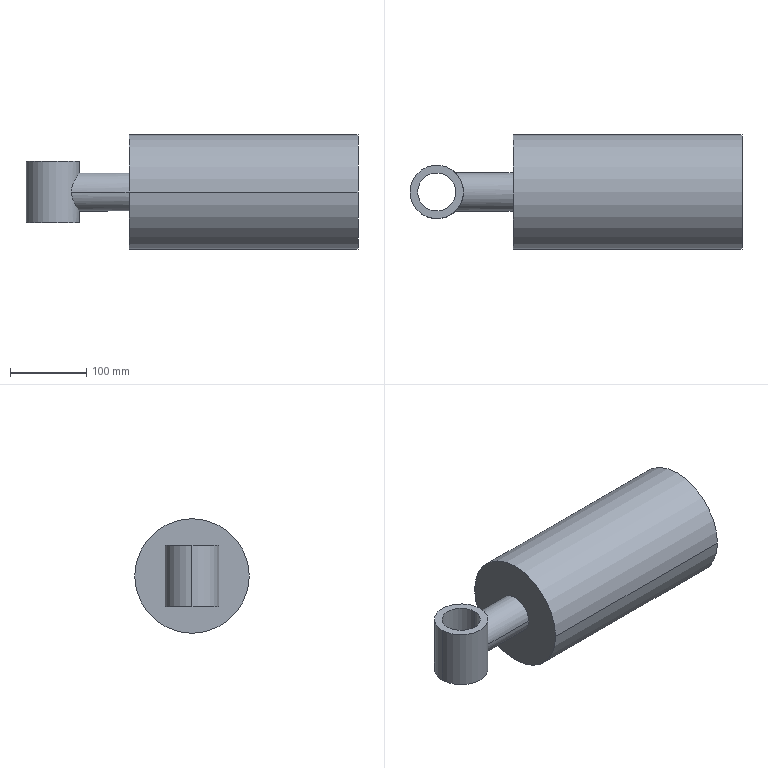Part | SolidWorks | 1 solid | 18 faces | box 435 x 150 x 150 mm | volume 3088587 mm3 | cylinder 12 | plane 6 | commonest cylinder face diameters 50 x4 40 x2 70 x2 110 x2 150 x2
STEP:
#1=CARTESIAN_POINT('',(400.,-75.,0.));
#2=VERTEX_POINT('',#1);
#3=CARTESIAN_POINT('',(400.,75.,0.));
#4=VERTEX_POINT('',#3);
#5=CARTESIAN_POINT('',(400.,0.,0.));
#6=DIRECTION('',(-1.,0.,0.));
#7=DIRECTION('',(0.,-1.,0.));
#8=AXIS2_PLACEMENT_3D('',#5,#6,#7);
#9=CIRCLE('',#8,75.);
#10=EDGE_CURVE('',#2,#4,#9,.T.);
#11=ORIENTED_EDGE('',*,*,#10,.T.);
#12=CARTESIAN_POINT('',(100.,75.,0.));
#13=VERTEX_POINT('',#12);
#14=CARTESIAN_POINT('',(0.,75.,0.));
#15=DIRECTION('',(-1.,0.,0.));
#16=VECTOR('',#15,1000.);
#17=LINE('',#14,#16);
#18=EDGE_CURVE('',#4,#13,#17,.T.);
#19=ORIENTED_EDGE('',*,*,#18,.T.);
#20=CARTESIAN_POINT('',(100.,-75.,0.));
#21=VERTEX_POINT('',#20);
#22=CARTESIAN_POINT('',(100.,0.,0.));
#23=DIRECTION('',(-1.,0.,0.));
#24=DIRECTION('',(0.,-1.,0.));
#25=AXIS2_PLACEMENT_3D('',#22,#23,#24);
#26=CIRCLE('',#25,75.);
#27=EDGE_CURVE('',#21,#13,#26,.T.);
#28=ORIENTED_EDGE('',*,*,#27,.F.);
#29=CARTESIAN_POINT('',(0.,-75.,0.));
#30=DIRECTION('',(-1.,0.,0.));
#31=VECTOR('',#30,1000.);
#32=LINE('',#29,#31);
#33=EDGE_CURVE('',#2,#21,#32,.T.);
#34=ORIENTED_EDGE('',*,*,#33,.F.);
#35=EDGE_LOOP('',(#11,#19,#28,#34));
#36=FACE_OUTER_BOUND('',#35,.T.);
#37=CARTESIAN_POINT('',(0.,0.,0.));
#38=DIRECTION('',(-1.,0.,0.));
#39=DIRECTION('',(0.,-1.,0.));
#40=AXIS2_PLACEMENT_3D('',#37,#38,#39);
#41=CYLINDRICAL_SURFACE('',#40,75.);
#42=ADVANCED_FACE('',(#36),#41,.T.);
#43=CARTESIAN_POINT('',(400.,20.,0.));
#44=VERTEX_POINT('',#43);
#45=CARTESIAN_POINT('',(400.,-20.,0.));
#46=VERTEX_POINT('',#45);
#47=CARTESIAN_POINT('',(400.,0.,0.));
#48=DIRECTION('',(-1.,0.,0.));
#49=DIRECTION('',(0.,-1.,0.));
#50=AXIS2_PLACEMENT_3D('',#47,#48,#49);
#51=CIRCLE('',#50,20.);
#52=EDGE_CURVE('',#44,#46,#51,.T.);
#53=ORIENTED_EDGE('',*,*,#52,.F.);
#54=CARTESIAN_POINT('',(380.,20.,0.));
#55=VERTEX_POINT('',#54);
#56=CARTESIAN_POINT('',(0.,20.,0.));
#57=DIRECTION('',(-1.,0.,0.));
#58=VECTOR('',#57,1000.);
#59=LINE('',#56,#58);
#60=EDGE_CURVE('',#44,#55,#59,.T.);
#61=ORIENTED_EDGE('',*,*,#60,.T.);
#62=CARTESIAN_POINT('',(380.,-20.,0.));
#63=VERTEX_POINT('',#62);
#64=CARTESIAN_POINT('',(380.,0.,0.));
#65=DIRECTION('',(-1.,0.,0.));
#66=DIRECTION('',(0.,-1.,0.));
#67=AXIS2_PLACEMENT_3D('',#64,#65,#66);
#68=CIRCLE('',#67,20.);
#69=EDGE_CURVE('',#55,#63,#68,.T.);
#70=ORIENTED_EDGE('',*,*,#69,.T.);
#71=CARTESIAN_POINT('',(0.,-20.,0.));
#72=DIRECTION('',(-1.,0.,0.));
#73=VECTOR('',#72,1000.);
#74=LINE('',#71,#73);
#75=EDGE_CURVE('',#46,#63,#74,.T.);
#76=ORIENTED_EDGE('',*,*,#75,.F.);
#77=EDGE_LOOP('',(#53,#61,#70,#76));
#78=FACE_OUTER_BOUND('',#77,.T.);
#79=CARTESIAN_POINT('',(0.,0.,0.));
#80=DIRECTION('',(-1.,0.,0.));
#81=DIRECTION('',(0.,-1.,0.));
#82=AXIS2_PLACEMENT_3D('',#79,#80,#81);
#83=CYLINDRICAL_SURFACE('',#82,20.);
#84=ADVANCED_FACE('',(#78),#83,.F.);
#85=CARTESIAN_POINT('',(380.,55.,0.));
#86=VERTEX_POINT('',#85);
#87=CARTESIAN_POINT('',(380.,-55.,0.));
#88=VERTEX_POINT('',#87);
#89=CARTESIAN_POINT('',(380.,0.,0.));
#90=DIRECTION('',(-1.,0.,0.));
#91=DIRECTION('',(0.,-1.,0.));
#92=AXIS2_PLACEMENT_3D('',#89,#90,#91);
#93=CIRCLE('',#92,55.);
#94=EDGE_CURVE('',#86,#88,#93,.T.);
#95=ORIENTED_EDGE('',*,*,#94,.F.);
#96=CARTESIAN_POINT('',(120.,55.,0.));
#97=VERTEX_POINT('',#96);
#98=CARTESIAN_POINT('',(0.,55.,0.));
#99=DIRECTION('',(-1.,0.,0.));
#100=VECTOR('',#99,1000.);
#101=LINE('',#98,#100);
#102=EDGE_CURVE('',#86,#97,#101,.T.);
#103=ORIENTED_EDGE('',*,*,#102,.T.);
#104=CARTESIAN_POINT('',(120.,-55.,0.));
#105=VERTEX_POINT('',#104);
#106=CARTESIAN_POINT('',(120.,0.,0.));
#107=DIRECTION('',(-1.,0.,0.));
#108=DIRECTION('',(0.,-1.,0.));
#109=AXIS2_PLACEMENT_3D('',#106,#107,#108);
#110=CIRCLE('',#109,55.);
#111=EDGE_CURVE('',#97,#105,#110,.T.);
#112=ORIENTED_EDGE('',*,*,#111,.T.);
#113=CARTESIAN_POINT('',(0.,-55.,0.));
#114=DIRECTION('',(-1.,0.,0.));
#115=VECTOR('',#114,1000.);
#116=LINE('',#113,#115);
#117=EDGE_CURVE('',#88,#105,#116,.T.);
#118=ORIENTED_EDGE('',*,*,#117,.F.);
#119=EDGE_LOOP('',(#95,#103,#112,#118));
#120=FACE_OUTER_BOUND('',#119,.T.);
#121=CARTESIAN_POINT('',(0.,0.,0.));
#122=DIRECTION('',(-1.,0.,0.));
#123=DIRECTION('',(0.,-1.,0.));
#124=AXIS2_PLACEMENT_3D('',#121,#122,#123);
#125=CYLINDRICAL_SURFACE('',#124,55.);
#126=ADVANCED_FACE('',(#120),#125,.F.);
#127=CARTESIAN_POINT('',(100.,-25.,0.));
#128=VERTEX_POINT('',#127);
#129=CARTESIAN_POINT('',(100.,25.,0.));
#130=VERTEX_POINT('',#129);
#131=CARTESIAN_POINT('',(100.,0.,0.));
#132=DIRECTION('',(-1.,0.,0.));
#133=DIRECTION('',(0.,-1.,0.));
#134=AXIS2_PLACEMENT_3D('',#131,#132,#133);
#135=CIRCLE('',#134,25.);
#136=EDGE_CURVE('',#128,#130,#135,.T.);
#137=ORIENTED_EDGE('',*,*,#136,.T.);
#138=CARTESIAN_POINT('',(24.495,25.,0.));
#139=VERTEX_POINT('',#138);
#140=CARTESIAN_POINT('',(0.,25.,0.));
#141=DIRECTION('',(-1.,0.,0.));
#142=VECTOR('',#141,1000.);
#143=LINE('',#140,#142);
#144=EDGE_CURVE('',#130,#139,#143,.T.);
#145=ORIENTED_EDGE('',*,*,#144,.T.);
#146=CARTESIAN_POINT('',(35.,0.,25.));
#147=VERTEX_POINT('',#146);
#148=CARTESIAN_POINT('',(24.495,25.,0.));
#149=CARTESIAN_POINT('',(24.495,25.,0.8465));
#150=CARTESIAN_POINT('',(24.539,24.957,1.695));
#151=CARTESIAN_POINT('',(24.671,24.826,2.973));
#152=CARTESIAN_POINT('',(24.726,24.772,3.398));
#153=CARTESIAN_POINT('',(24.855,24.642,4.235));
#154=CARTESIAN_POINT('',(24.929,24.567,4.649));
#155=CARTESIAN_POINT('',(25.178,24.313,5.879));
#156=CARTESIAN_POINT('',(25.379,24.105,6.682));
#157=CARTESIAN_POINT('',(25.838,23.612,8.257));
#158=CARTESIAN_POINT('',(26.097,23.326,9.031));
#159=CARTESIAN_POINT('',(26.925,22.377,11.264));
#160=CARTESIAN_POINT('',(27.546,21.62,12.651));
#161=CARTESIAN_POINT('',(28.516,20.301,14.612));
#162=CARTESIAN_POINT('',(28.847,19.829,15.245));
#163=CARTESIAN_POINT('',(29.513,18.825,16.47));
#164=CARTESIAN_POINT('',(29.844,18.297,17.054));
#165=CARTESIAN_POINT('',(30.82,16.636,18.728));
#166=CARTESIAN_POINT('',(31.451,15.426,19.739));
#167=CARTESIAN_POINT('',(32.327,13.436,21.098));
#168=CARTESIAN_POINT('',(32.608,12.74,21.526));
#169=CARTESIAN_POINT('',(33.13,11.312,22.309));
#170=CARTESIAN_POINT('',(33.372,10.579,22.666));
#171=CARTESIAN_POINT('',(33.814,9.07,23.311));
#172=CARTESIAN_POINT('',(34.013,8.294,23.599));
#173=CARTESIAN_POINT('',(34.363,6.698,24.1));
#174=CARTESIAN_POINT('',(34.514,5.872,24.315));
#175=CARTESIAN_POINT('',(34.876,3.386,24.827));
#176=CARTESIAN_POINT('',(35.,1.705,25.));
#177=CARTESIAN_POINT('',(35.,0.,25.));
#178=B_SPLINE_CURVE_WITH_KNOTS('',3,(#148,#149,#150,#151,#152,#153,#154,#155,#156,#157,#158,#159,#160,#161,#162,#163,#164,#165,#166,#167,#168,#169,#170,#171,#172,#173,#174,#175,#176,#177),.UNSPECIFIED.,.F.,.F.,(4,2,2,2,2,2,2,2,2,2,2,2,2,2,4),(0.08125,0.08378,0.08505,0.08632,0.08886,0.09139,0.09647,0.099,0.1015,0.1066,0.1091,0.1117,0.1142,0.1168,0.1218),.UNSPECIFIED.);
#179=EDGE_CURVE('',#139,#147,#178,.T.);
#180=ORIENTED_EDGE('',*,*,#179,.T.);
#181=CARTESIAN_POINT('',(24.495,-25.,0.));
#182=VERTEX_POINT('',#181);
#183=CARTESIAN_POINT('',(35.,0.,25.));
#184=CARTESIAN_POINT('',(35.,-0.4259,25.));
#185=CARTESIAN_POINT('',(34.992,-0.8533,24.989));
#186=CARTESIAN_POINT('',(34.961,-1.711,24.945));
#187=CARTESIAN_POINT('',(34.937,-2.14,24.912));
#188=CARTESIAN_POINT('',(34.844,-3.414,24.781));
#189=CARTESIAN_POINT('',(34.751,-4.25,24.651));
#190=CARTESIAN_POINT('',(34.51,-5.897,24.309));
#191=CARTESIAN_POINT('',(34.361,-6.709,24.098));
#192=CARTESIAN_POINT('',(34.097,-7.908,23.72));
#193=CARTESIAN_POINT('',(34.003,-8.306,23.584));
#194=CARTESIAN_POINT('',(33.802,-9.088,23.293));
#195=CARTESIAN_POINT('',(33.696,-9.473,23.139));
#196=CARTESIAN_POINT('',(33.14,-11.367,22.327));
#197=CARTESIAN_POINT('',(32.614,-12.786,21.544));
#198=CARTESIAN_POINT('',(31.733,-14.784,20.177));
#199=CARTESIAN_POINT('',(31.426,-15.422,19.692));
#200=CARTESIAN_POINT('',(30.8,-16.639,18.676));
#201=CARTESIAN_POINT('',(30.478,-17.219,18.142));
#202=CARTESIAN_POINT('',(29.827,-18.325,17.024));
#203=CARTESIAN_POINT('',(29.496,-18.851,16.44));
#204=CARTESIAN_POINT('',(28.833,-19.85,15.218));
#205=CARTESIAN_POINT('',(28.5,-20.323,14.58));
#206=CARTESIAN_POINT('',(27.53,-21.641,12.616));
#207=CARTESIAN_POINT('',(26.912,-22.393,11.231));
#208=CARTESIAN_POINT('',(26.091,-23.333,9.012));
#209=CARTESIAN_POINT('',(25.836,-23.614,8.249));
#210=CARTESIAN_POINT('',(25.49,-23.985,7.063));
#211=CARTESIAN_POINT('',(25.381,-24.1,6.661));
#212=CARTESIAN_POINT('',(25.182,-24.308,5.855));
#213=CARTESIAN_POINT('',(25.091,-24.402,5.45));
#214=CARTESIAN_POINT('',(24.844,-24.655,4.224));
#215=CARTESIAN_POINT('',(24.715,-24.783,3.397));
#216=CARTESIAN_POINT('',(24.584,-24.912,2.137));
#217=CARTESIAN_POINT('',(24.551,-24.945,1.714));
#218=CARTESIAN_POINT('',(24.506,-24.989,0.8617));
#219=CARTESIAN_POINT('',(24.495,-25.,0.4306));
#220=CARTESIAN_POINT('',(24.495,-25.,0.));
#221=B_SPLINE_CURVE_WITH_KNOTS('',3,(#183,#184,#185,#186,#187,#188,#189,#190,#191,#192,#193,#194,#195,#196,#197,#198,#199,#200,#201,#202,#203,#204,#205,#206,#207,#208,#209,#210,#211,#212,#213,#214,#215,#216,#217,#218,#219,#220),.UNSPECIFIED.,.F.,.F.,(4,2,2,2,2,2,2,2,2,2,2,2,2,2,2,2,2,2,4),(0.1218,0.1231,0.1244,0.1269,0.1294,0.1307,0.132,0.137,0.1396,0.1421,0.1446,0.1472,0.1522,0.1548,0.156,0.1573,0.1598,0.1611,0.1624),.UNSPECIFIED.);
#222=EDGE_CURVE('',#147,#182,#221,.T.);
#223=ORIENTED_EDGE('',*,*,#222,.T.);
#224=CARTESIAN_POINT('',(0.,-25.,0.));
#225=DIRECTION('',(-1.,0.,0.));
#226=VECTOR('',#225,1000.);
#227=LINE('',#224,#226);
#228=EDGE_CURVE('',#128,#182,#227,.T.);
#229=ORIENTED_EDGE('',*,*,#228,.F.);
#230=EDGE_LOOP('',(#137,#145,#180,#223,#229));
#231=FACE_OUTER_BOUND('',#230,.T.);
#232=CARTESIAN_POINT('',(0.,0.,0.));
#233=DIRECTION('',(-1.,0.,0.));
#234=DIRECTION('',(0.,-1.,0.));
#235=AXIS2_PLACEMENT_3D('',#232,#233,#234);
#236=CYLINDRICAL_SURFACE('',#235,25.);
#237=ADVANCED_FACE('',(#231),#236,.T.);
#238=CARTESIAN_POINT('',(-25.,0.,40.));
#239=VERTEX_POINT('',#238);
#240=CARTESIAN_POINT('',(25.,0.,40.));
#241=VERTEX_POINT('',#240);
#242=CARTESIAN_POINT('',(0.,0.,40.));
#243=DIRECTION('',(0.,0.,1.));
#244=DIRECTION('',(1.,0.,0.));
#245=AXIS2_PLACEMENT_3D('',#242,#243,#244);
#246=CIRCLE('',#245,25.);
#247=EDGE_CURVE('',#239,#241,#246,.T.);
#248=ORIENTED_EDGE('',*,*,#247,.T.);
#249=CARTESIAN_POINT('',(25.,0.,-40.));
#250=VERTEX_POINT('',#249);
#251=CARTESIAN_POINT('',(25.,0.,40.));
#252=DIRECTION('',(0.,0.,-1.));
#253=VECTOR('',#252,1000.);
#254=LINE('',#251,#253);
#255=EDGE_CURVE('',#241,#250,#254,.T.);
#256=ORIENTED_EDGE('',*,*,#255,.T.);
#257=CARTESIAN_POINT('',(-25.,0.,-40.));
#258=VERTEX_POINT('',#257);
#259=CARTESIAN_POINT('',(0.,0.,-40.));
#260=DIRECTION('',(0.,0.,1.));
#261=DIRECTION('',(1.,0.,0.));
#262=AXIS2_PLACEMENT_3D('',#259,#260,#261);
#263=CIRCLE('',#262,25.);
#264=EDGE_CURVE('',#258,#250,#263,.T.);
#265=ORIENTED_EDGE('',*,*,#264,.F.);
#266=CARTESIAN_POINT('',(-25.,0.,40.));
#267=DIRECTION('',(0.,0.,-1.));
#268=VECTOR('',#267,1000.);
#269=LINE('',#266,#268);
#270=EDGE_CURVE('',#239,#258,#269,.T.);
#271=ORIENTED_EDGE('',*,*,#270,.F.);
#272=EDGE_LOOP('',(#248,#256,#265,#271));
#273=FACE_OUTER_BOUND('',#272,.T.);
#274=CARTESIAN_POINT('',(0.,0.,40.));
#275=DIRECTION('',(0.,0.,-1.));
#276=DIRECTION('',(-1.,0.,0.));
#277=AXIS2_PLACEMENT_3D('',#274,#275,#276);
#278=CYLINDRICAL_SURFACE('',#277,25.);
#279=ADVANCED_FACE('',(#273),#278,.F.);
#280=CARTESIAN_POINT('',(35.,0.,40.));
#281=VERTEX_POINT('',#280);
#282=CARTESIAN_POINT('',(-35.,0.,40.));
#283=VERTEX_POINT('',#282);
#284=CARTESIAN_POINT('',(0.,0.,40.));
#285=DIRECTION('',(0.,0.,1.));
#286=DIRECTION('',(1.,0.,0.));
#287=AXIS2_PLACEMENT_3D('',#284,#285,#286);
#288=CIRCLE('',#287,35.);
#289=EDGE_CURVE('',#281,#283,#288,.T.);
#290=ORIENTED_EDGE('',*,*,#289,.F.);
#291=CARTESIAN_POINT('',(35.,0.,40.));
#292=DIRECTION('',(0.,0.,-1.));
#293=VECTOR('',#292,1000.);
#294=LINE('',#291,#293);
#295=EDGE_CURVE('',#281,#147,#294,.T.);
#296=ORIENTED_EDGE('',*,*,#295,.T.);
#297=ORIENTED_EDGE('',*,*,#179,.F.);
#298=CARTESIAN_POINT('',(35.,0.,-25.));
#299=VERTEX_POINT('',#298);
#300=CARTESIAN_POINT('',(35.,0.,-25.));
#301=CARTESIAN_POINT('',(35.,1.707,-25.));
#302=CARTESIAN_POINT('',(34.876,3.392,-24.827));
#303=CARTESIAN_POINT('',(34.573,5.47,-24.398));
#304=CARTESIAN_POINT('',(34.504,5.885,-24.301));
#305=CARTESIAN_POINT('',(34.355,6.702,-24.089));
#306=CARTESIAN_POINT('',(34.274,7.106,-23.973));
#307=CARTESIAN_POINT('',(34.011,8.3,-23.597));
#308=CARTESIAN_POINT('',(33.812,9.076,-23.309));
#309=CARTESIAN_POINT('',(33.369,10.589,-22.662));
#310=CARTESIAN_POINT('',(33.125,11.327,-22.302));
#311=CARTESIAN_POINT('',(32.599,12.762,-21.513));
#312=CARTESIAN_POINT('',(32.321,13.449,-21.089));
#313=CARTESIAN_POINT('',(31.447,15.432,-19.733));
#314=CARTESIAN_POINT('',(30.814,16.648,-18.718));
#315=CARTESIAN_POINT('',(29.498,18.882,-16.462));
#316=CARTESIAN_POINT('',(28.832,19.873,-15.249));
#317=CARTESIAN_POINT('',(27.864,21.187,-13.294));
#318=CARTESIAN_POINT('',(27.547,21.596,-12.619));
#319=CARTESIAN_POINT('',(26.934,22.356,-11.217));
#320=CARTESIAN_POINT('',(26.636,22.709,-10.487));
#321=CARTESIAN_POINT('',(25.81,23.655,-8.25));
#322=CARTESIAN_POINT('',(25.341,24.147,-6.691));
#323=CARTESIAN_POINT('',(24.926,24.571,-4.631));
#324=CARTESIAN_POINT('',(24.851,24.646,-4.212));
#325=CARTESIAN_POINT('',(24.723,24.775,-3.373));
#326=CARTESIAN_POINT('',(24.669,24.829,-2.953));
#327=CARTESIAN_POINT('',(24.539,24.957,-1.69));
#328=CARTESIAN_POINT('',(24.495,25.,-0.8465));
#329=CARTESIAN_POINT('',(24.495,25.,0.));
#330=B_SPLINE_CURVE_WITH_KNOTS('',3,(#300,#301,#302,#303,#304,#305,#306,#307,#308,#309,#310,#311,#312,#313,#314,#315,#316,#317,#318,#319,#320,#321,#322,#323,#324,#325,#326,#327,#328,#329),.UNSPECIFIED.,.F.,.F.,(4,2,2,2,2,2,2,2,2,2,2,2,2,2,4),(0.04066,0.04573,0.047,0.04827,0.0508,0.05334,0.05588,0.06095,0.06602,0.06856,0.0711,0.07617,0.07744,0.07871,0.08125),.UNSPECIFIED.);
#331=EDGE_CURVE('',#299,#139,#330,.T.);
#332=ORIENTED_EDGE('',*,*,#331,.F.);
#333=CARTESIAN_POINT('',(35.,0.,-40.));
#334=VERTEX_POINT('',#333);
#335=CARTESIAN_POINT('',(35.,0.,40.));
#336=DIRECTION('',(0.,0.,-1.));
#337=VECTOR('',#336,1000.);
#338=LINE('',#335,#337);
#339=EDGE_CURVE('',#299,#334,#338,.T.);
#340=ORIENTED_EDGE('',*,*,#339,.T.);
#341=CARTESIAN_POINT('',(-35.,0.,-40.));
#342=VERTEX_POINT('',#341);
#343=CARTESIAN_POINT('',(0.,0.,-40.));
#344=DIRECTION('',(0.,0.,1.));
#345=DIRECTION('',(1.,0.,0.));
#346=AXIS2_PLACEMENT_3D('',#343,#344,#345);
#347=CIRCLE('',#346,35.);
#348=EDGE_CURVE('',#334,#342,#347,.T.);
#349=ORIENTED_EDGE('',*,*,#348,.T.);
#350=CARTESIAN_POINT('',(-35.,0.,40.));
#351=DIRECTION('',(0.,0.,-1.));
#352=VECTOR('',#351,1000.);
#353=LINE('',#350,#352);
#354=EDGE_CURVE('',#283,#342,#353,.T.);
#355=ORIENTED_EDGE('',*,*,#354,.F.);
#356=EDGE_LOOP('',(#290,#296,#297,#332,#340,#349,#355));
#357=FACE_OUTER_BOUND('',#356,.T.);
#358=CARTESIAN_POINT('',(0.,0.,40.));
#359=DIRECTION('',(0.,0.,-1.));
#360=DIRECTION('',(-1.,0.,0.));
#361=AXIS2_PLACEMENT_3D('',#358,#359,#360);
#362=CYLINDRICAL_SURFACE('',#361,35.);
#363=ADVANCED_FACE('',(#357),#362,.T.);
#364=ORIENTED_EDGE('',*,*,#295,.F.);
#365=CARTESIAN_POINT('',(0.,0.,40.));
#366=DIRECTION('',(0.,0.,1.));
#367=DIRECTION('',(1.,0.,0.));
#368=AXIS2_PLACEMENT_3D('',#365,#366,#367);
#369=CIRCLE('',#368,35.);
#370=EDGE_CURVE('',#283,#281,#369,.T.);
#371=ORIENTED_EDGE('',*,*,#370,.F.);
#372=ORIENTED_EDGE('',*,*,#354,.T.);
#373=CARTESIAN_POINT('',(0.,0.,-40.));
#374=DIRECTION('',(0.,0.,1.));
#375=DIRECTION('',(1.,0.,0.));
#376=AXIS2_PLACEMENT_3D('',#373,#374,#375);
#377=CIRCLE('',#376,35.);
#378=EDGE_CURVE('',#342,#334,#377,.T.);
#379=ORIENTED_EDGE('',*,*,#378,.T.);
#380=ORIENTED_EDGE('',*,*,#339,.F.);
#381=CARTESIAN_POINT('',(24.495,-25.,0.));
#382=CARTESIAN_POINT('',(24.495,-25.,-1.727));
#383=CARTESIAN_POINT('',(24.678,-24.823,-3.404));
#384=CARTESIAN_POINT('',(25.09,-24.403,-5.446));
#385=CARTESIAN_POINT('',(25.181,-24.309,-5.851));
#386=CARTESIAN_POINT('',(25.381,-24.101,-6.658));
#387=CARTESIAN_POINT('',(25.489,-23.986,-7.059));
#388=CARTESIAN_POINT('',(25.834,-23.616,-8.244));
#389=CARTESIAN_POINT('',(26.09,-23.335,-9.008));
#390=CARTESIAN_POINT('',(26.639,-22.705,-10.493));
#391=CARTESIAN_POINT('',(26.933,-22.358,-11.214));
#392=CARTESIAN_POINT('',(27.546,-21.597,-12.617));
#393=CARTESIAN_POINT('',(27.868,-21.182,-13.302));
#394=CARTESIAN_POINT('',(28.843,-19.857,-15.271));
#395=CARTESIAN_POINT('',(29.51,-18.863,-16.482));
#396=CARTESIAN_POINT('',(30.326,-17.476,-17.881));
#397=CARTESIAN_POINT('',(30.489,-17.192,-18.155));
#398=CARTESIAN_POINT('',(30.811,-16.607,-18.691));
#399=CARTESIAN_POINT('',(30.971,-16.306,-18.954));
#400=CARTESIAN_POINT('',(31.444,-15.387,-19.72));
#401=CARTESIAN_POINT('',(31.747,-14.752,-20.199));
#402=CARTESIAN_POINT('',(32.616,-12.779,-21.546));
#403=CARTESIAN_POINT('',(33.138,-11.373,-22.324));
#404=CARTESIAN_POINT('',(33.693,-9.484,-23.135));
#405=CARTESIAN_POINT('',(33.799,-9.1,-23.289));
#406=CARTESIAN_POINT('',(34.,-8.318,-23.579));
#407=CARTESIAN_POINT('',(34.095,-7.919,-23.716));
#408=CARTESIAN_POINT('',(34.359,-6.718,-24.095));
#409=CARTESIAN_POINT('',(34.508,-5.905,-24.307));
#410=CARTESIAN_POINT('',(34.75,-4.256,-24.649));
#411=CARTESIAN_POINT('',(34.843,-3.419,-24.78));
#412=CARTESIAN_POINT('',(34.968,-1.721,-24.955));
#413=CARTESIAN_POINT('',(35.,-0.8551,-25.));
#414=CARTESIAN_POINT('',(35.,0.,-25.));
#415=B_SPLINE_CURVE_WITH_KNOTS('',3,(#381,#382,#383,#384,#385,#386,#387,#388,#389,#390,#391,#392,#393,#394,#395,#396,#397,#398,#399,#400,#401,#402,#403,#404,#405,#406,#407,#408,#409,#410,#411,#412,#413,#414),.UNSPECIFIED.,.F.,.F.,(4,2,2,2,2,2,2,2,2,2,2,2,2,2,2,2,4),(0.,0.005082,0.006352,0.007623,0.01016,0.0127,0.01525,0.02033,0.0216,0.02287,0.02541,0.03049,0.03176,0.03303,0.03557,0.03811,0.04066),.UNSPECIFIED.);
#416=EDGE_CURVE('',#182,#299,#415,.T.);
#417=ORIENTED_EDGE('',*,*,#416,.F.);
#418=ORIENTED_EDGE('',*,*,#222,.F.);
#419=EDGE_LOOP('',(#364,#371,#372,#379,#380,#417,#418));
#420=FACE_OUTER_BOUND('',#419,.T.);
#421=CARTESIAN_POINT('',(0.,0.,40.));
#422=DIRECTION('',(0.,0.,-1.));
#423=DIRECTION('',(-1.,0.,0.));
#424=AXIS2_PLACEMENT_3D('',#421,#422,#423);
#425=CYLINDRICAL_SURFACE('',#424,35.);
#426=ADVANCED_FACE('',(#420),#425,.T.);
#427=ORIENTED_EDGE('',*,*,#255,.F.);
#428=CARTESIAN_POINT('',(0.,0.,40.));
#429=DIRECTION('',(0.,0.,1.));
#430=DIRECTION('',(1.,0.,0.));
#431=AXIS2_PLACEMENT_3D('',#428,#429,#430);
#432=CIRCLE('',#431,25.);
#433=EDGE_CURVE('',#241,#239,#432,.T.);
#434=ORIENTED_EDGE('',*,*,#433,.T.);
#435=ORIENTED_EDGE('',*,*,#270,.T.);
#436=CARTESIAN_POINT('',(0.,0.,-40.));
#437=DIRECTION('',(0.,0.,1.));
#438=DIRECTION('',(1.,0.,0.));
#439=AXIS2_PLACEMENT_3D('',#436,#437,#438);
#440=CIRCLE('',#439,25.);
#441=EDGE_CURVE('',#250,#258,#440,.T.);
#442=ORIENTED_EDGE('',*,*,#441,.F.);
#443=EDGE_LOOP('',(#427,#434,#435,#442));
#444=FACE_OUTER_BOUND('',#443,.T.);
#445=CARTESIAN_POINT('',(0.,0.,40.));
#446=DIRECTION('',(0.,0.,-1.));
#447=DIRECTION('',(-1.,0.,0.));
#448=AXIS2_PLACEMENT_3D('',#445,#446,#447);
#449=CYLINDRICAL_SURFACE('',#448,25.);
#450=ADVANCED_FACE('',(#444),#449,.F.);
#451=ORIENTED_EDGE('',*,*,#370,.T.);
#452=ORIENTED_EDGE('',*,*,#289,.T.);
#453=EDGE_LOOP('',(#451,#452));
#454=FACE_OUTER_BOUND('',#453,.T.);
#455=ORIENTED_EDGE('',*,*,#247,.F.);
#456=ORIENTED_EDGE('',*,*,#433,.F.);
#457=EDGE_LOOP('',(#455,#456));
#458=FACE_BOUND('',#457,.T.);
#459=CARTESIAN_POINT('',(0.,0.,40.));
#460=DIRECTION('',(0.,0.,1.));
#461=DIRECTION('',(1.,0.,0.));
#462=AXIS2_PLACEMENT_3D('',#459,#460,#461);
#463=PLANE('',#462);
#464=ADVANCED_FACE('',(#454,#458),#463,.T.);
#465=ORIENTED_EDGE('',*,*,#378,.F.);
#466=ORIENTED_EDGE('',*,*,#348,.F.);
#467=EDGE_LOOP('',(#465,#466));
#468=FACE_OUTER_BOUND('',#467,.T.);
#469=ORIENTED_EDGE('',*,*,#264,.T.);
#470=ORIENTED_EDGE('',*,*,#441,.T.);
#471=EDGE_LOOP('',(#469,#470));
#472=FACE_BOUND('',#471,.T.);
#473=CARTESIAN_POINT('',(0.,0.,-40.));
#474=DIRECTION('',(0.,0.,1.));
#475=DIRECTION('',(1.,0.,0.));
#476=AXIS2_PLACEMENT_3D('',#473,#474,#475);
#477=PLANE('',#476);
#478=ADVANCED_FACE('',(#468,#472),#477,.F.);
#479=ORIENTED_EDGE('',*,*,#144,.F.);
#480=CARTESIAN_POINT('',(100.,0.,0.));
#481=DIRECTION('',(-1.,0.,0.));
#482=DIRECTION('',(0.,-1.,0.));
#483=AXIS2_PLACEMENT_3D('',#480,#481,#482);
#484=CIRCLE('',#483,25.);
#485=EDGE_CURVE('',#130,#128,#484,.T.);
#486=ORIENTED_EDGE('',*,*,#485,.T.);
#487=ORIENTED_EDGE('',*,*,#228,.T.);
#488=ORIENTED_EDGE('',*,*,#416,.T.);
#489=ORIENTED_EDGE('',*,*,#331,.T.);
#490=EDGE_LOOP('',(#479,#486,#487,#488,#489));
#491=FACE_OUTER_BOUND('',#490,.T.);
#492=CARTESIAN_POINT('',(0.,0.,0.));
#493=DIRECTION('',(-1.,0.,0.));
#494=DIRECTION('',(0.,-1.,0.));
#495=AXIS2_PLACEMENT_3D('',#492,#493,#494);
#496=CYLINDRICAL_SURFACE('',#495,25.);
#497=ADVANCED_FACE('',(#491),#496,.T.);
#498=CARTESIAN_POINT('',(120.,0.,0.));
#499=DIRECTION('',(-1.,0.,0.));
#500=DIRECTION('',(0.,-1.,0.));
#501=AXIS2_PLACEMENT_3D('',#498,#499,#500);
#502=CIRCLE('',#501,55.);
#503=EDGE_CURVE('',#105,#97,#502,.T.);
#504=ORIENTED_EDGE('',*,*,#503,.F.);
#505=ORIENTED_EDGE('',*,*,#111,.F.);
#506=EDGE_LOOP('',(#504,#505));
#507=FACE_OUTER_BOUND('',#506,.T.);
#508=CARTESIAN_POINT('',(120.,0.,0.));
#509=DIRECTION('',(-1.,0.,0.));
#510=DIRECTION('',(0.,-1.,0.));
#511=AXIS2_PLACEMENT_3D('',#508,#509,#510);
#512=PLANE('',#511);
#513=ADVANCED_FACE('',(#507),#512,.F.);
#514=ORIENTED_EDGE('',*,*,#102,.F.);
#515=CARTESIAN_POINT('',(380.,0.,0.));
#516=DIRECTION('',(-1.,0.,0.));
#517=DIRECTION('',(0.,-1.,0.));
#518=AXIS2_PLACEMENT_3D('',#515,#516,#517);
#519=CIRCLE('',#518,55.);
#520=EDGE_CURVE('',#88,#86,#519,.T.);
#521=ORIENTED_EDGE('',*,*,#520,.F.);
#522=ORIENTED_EDGE('',*,*,#117,.T.);
#523=ORIENTED_EDGE('',*,*,#503,.T.);
#524=EDGE_LOOP('',(#514,#521,#522,#523));
#525=FACE_OUTER_BOUND('',#524,.T.);
#526=CARTESIAN_POINT('',(0.,0.,0.));
#527=DIRECTION('',(-1.,0.,0.));
#528=DIRECTION('',(0.,-1.,0.));
#529=AXIS2_PLACEMENT_3D('',#526,#527,#528);
#530=CYLINDRICAL_SURFACE('',#529,55.);
#531=ADVANCED_FACE('',(#525),#530,.F.);
#532=CARTESIAN_POINT('',(380.,0.,0.));
#533=DIRECTION('',(-1.,0.,0.));
#534=DIRECTION('',(0.,-1.,0.));
#535=AXIS2_PLACEMENT_3D('',#532,#533,#534);
#536=CIRCLE('',#535,20.);
#537=EDGE_CURVE('',#63,#55,#536,.T.);
#538=ORIENTED_EDGE('',*,*,#537,.F.);
#539=ORIENTED_EDGE('',*,*,#69,.F.);
#540=EDGE_LOOP('',(#538,#539));
#541=FACE_BOUND('',#540,.T.);
#542=ORIENTED_EDGE('',*,*,#520,.T.);
#543=ORIENTED_EDGE('',*,*,#94,.T.);
#544=EDGE_LOOP('',(#542,#543));
#545=FACE_OUTER_BOUND('',#544,.T.);
#546=CARTESIAN_POINT('',(380.,0.,0.));
#547=DIRECTION('',(1.,0.,0.));
#548=DIRECTION('',(0.,1.,0.));
#549=AXIS2_PLACEMENT_3D('',#546,#547,#548);
#550=PLANE('',#549);
#551=ADVANCED_FACE('',(#541,#545),#550,.F.);
#552=ORIENTED_EDGE('',*,*,#60,.F.);
#553=CARTESIAN_POINT('',(400.,0.,0.));
#554=DIRECTION('',(-1.,0.,0.));
#555=DIRECTION('',(0.,-1.,0.));
#556=AXIS2_PLACEMENT_3D('',#553,#554,#555);
#557=CIRCLE('',#556,20.);
#558=EDGE_CURVE('',#46,#44,#557,.T.);
#559=ORIENTED_EDGE('',*,*,#558,.F.);
#560=ORIENTED_EDGE('',*,*,#75,.T.);
#561=ORIENTED_EDGE('',*,*,#537,.T.);
#562=EDGE_LOOP('',(#552,#559,#560,#561));
#563=FACE_OUTER_BOUND('',#562,.T.);
#564=CARTESIAN_POINT('',(0.,0.,0.));
#565=DIRECTION('',(-1.,0.,0.));
#566=DIRECTION('',(0.,-1.,0.));
#567=AXIS2_PLACEMENT_3D('',#564,#565,#566);
#568=CYLINDRICAL_SURFACE('',#567,20.);
#569=ADVANCED_FACE('',(#563),#568,.F.);
#570=ORIENTED_EDGE('',*,*,#10,.F.);
#571=CARTESIAN_POINT('',(400.,0.,0.));
#572=DIRECTION('',(-1.,0.,0.));
#573=DIRECTION('',(0.,-1.,0.));
#574=AXIS2_PLACEMENT_3D('',#571,#572,#573);
#575=CIRCLE('',#574,75.);
#576=EDGE_CURVE('',#4,#2,#575,.T.);
#577=ORIENTED_EDGE('',*,*,#576,.F.);
#578=EDGE_LOOP('',(#570,#577));
#579=FACE_OUTER_BOUND('',#578,.T.);
#580=ORIENTED_EDGE('',*,*,#558,.T.);
#581=ORIENTED_EDGE('',*,*,#52,.T.);
#582=EDGE_LOOP('',(#580,#581));
#583=FACE_BOUND('',#582,.T.);
#584=CARTESIAN_POINT('',(400.,0.,0.));
#585=DIRECTION('',(-1.,0.,0.));
#586=DIRECTION('',(0.,-1.,0.));
#587=AXIS2_PLACEMENT_3D('',#584,#585,#586);
#588=PLANE('',#587);
#589=ADVANCED_FACE('',(#579,#583),#588,.F.);
#590=ORIENTED_EDGE('',*,*,#18,.F.);
#591=ORIENTED_EDGE('',*,*,#576,.T.);
#592=ORIENTED_EDGE('',*,*,#33,.T.);
#593=CARTESIAN_POINT('',(100.,0.,0.));
#594=DIRECTION('',(-1.,0.,0.));
#595=DIRECTION('',(0.,-1.,0.));
#596=AXIS2_PLACEMENT_3D('',#593,#594,#595);
#597=CIRCLE('',#596,75.);
#598=EDGE_CURVE('',#13,#21,#597,.T.);
#599=ORIENTED_EDGE('',*,*,#598,.F.);
#600=EDGE_LOOP('',(#590,#591,#592,#599));
#601=FACE_OUTER_BOUND('',#600,.T.);
#602=CARTESIAN_POINT('',(0.,0.,0.));
#603=DIRECTION('',(-1.,0.,0.));
#604=DIRECTION('',(0.,-1.,0.));
#605=AXIS2_PLACEMENT_3D('',#602,#603,#604);
#606=CYLINDRICAL_SURFACE('',#605,75.);
#607=ADVANCED_FACE('',(#601),#606,.T.);
#608=ORIENTED_EDGE('',*,*,#136,.F.);
#609=ORIENTED_EDGE('',*,*,#485,.F.);
#610=EDGE_LOOP('',(#608,#609));
#611=FACE_BOUND('',#610,.T.);
#612=ORIENTED_EDGE('',*,*,#27,.T.);
#613=ORIENTED_EDGE('',*,*,#598,.T.);
#614=EDGE_LOOP('',(#612,#613));
#615=FACE_OUTER_BOUND('',#614,.T.);
#616=CARTESIAN_POINT('',(100.,0.,0.));
#617=DIRECTION('',(1.,0.,0.));
#618=DIRECTION('',(0.,1.,0.));
#619=AXIS2_PLACEMENT_3D('',#616,#617,#618);
#620=PLANE('',#619);
#621=ADVANCED_FACE('',(#611,#615),#620,.F.);
#622=CLOSED_SHELL('',(#42,#84,#126,#237,#279,#363,#426,#450,#464,#478,#497,#513,#531,#551,#569,#589,#607,#621));
#623=MANIFOLD_SOLID_BREP('',#622);
#624=CARTESIAN_POINT('',(0.,0.,0.));
#625=DIRECTION('',(0.,0.,1.));
#626=DIRECTION('',(1.,0.,0.));
#627=AXIS2_PLACEMENT_3D('',#624,#625,#626);
#628=(LENGTH_UNIT()NAMED_UNIT(*)SI_UNIT(.MILLI.,.METRE.));
#629=UNCERTAINTY_MEASURE_WITH_UNIT(LENGTH_MEASURE(0.00001),#628,'','');
#630=(NAMED_UNIT(*)PLANE_ANGLE_UNIT()SI_UNIT($,.RADIAN.));
#631=(NAMED_UNIT(*)SI_UNIT($,.STERADIAN.)SOLID_ANGLE_UNIT());
#632=(GEOMETRIC_REPRESENTATION_CONTEXT(3)GLOBAL_UNCERTAINTY_ASSIGNED_CONTEXT((#629))GLOBAL_UNIT_ASSIGNED_CONTEXT((#628,#630,#631))REPRESENTATION_CONTEXT('',''));
#633=ADVANCED_BREP_SHAPE_REPRESENTATION('',(#623,#627),#632);